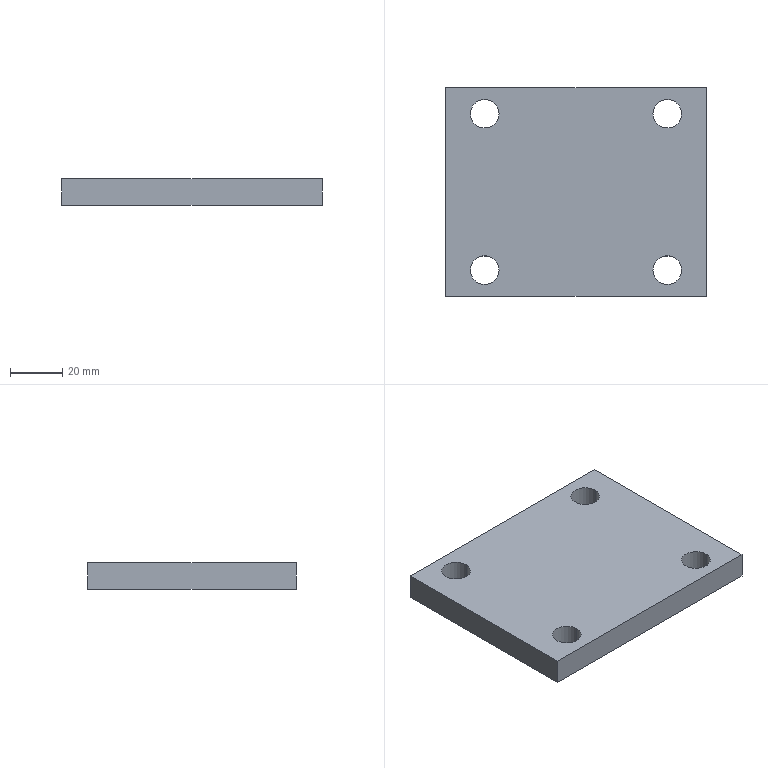Part | SolidWorks | features Extrusion 1 | 1 solid | 14 faces | box 100 x 80 x 10 mm | volume 76199 mm3 | cylinder 8 | plane 6 | commonest cylinder face diameters 11 x8
STEP:
#1=CARTESIAN_POINT('',(29.5,30.,10.));
#2=VERTEX_POINT('',#1);
#3=CARTESIAN_POINT('',(40.5,30.,10.));
#4=VERTEX_POINT('',#3);
#5=CARTESIAN_POINT('',(35.,30.,10.));
#6=DIRECTION('',(0.,0.,1.));
#7=DIRECTION('',(1.,0.,0.));
#8=AXIS2_PLACEMENT_3D('',#5,#6,#7);
#9=CIRCLE('',#8,5.5);
#10=EDGE_CURVE('',#2,#4,#9,.T.);
#11=ORIENTED_EDGE('',*,*,#10,.T.);
#12=CARTESIAN_POINT('',(40.5,30.,0.));
#13=VERTEX_POINT('',#12);
#14=CARTESIAN_POINT('',(40.5,30.,10.));
#15=DIRECTION('',(0.,0.,-1.));
#16=VECTOR('',#15,1000.);
#17=LINE('',#14,#16);
#18=EDGE_CURVE('',#4,#13,#17,.T.);
#19=ORIENTED_EDGE('',*,*,#18,.T.);
#20=CARTESIAN_POINT('',(29.5,30.,0.));
#21=VERTEX_POINT('',#20);
#22=CARTESIAN_POINT('',(35.,30.,0.));
#23=DIRECTION('',(0.,0.,1.));
#24=DIRECTION('',(1.,0.,0.));
#25=AXIS2_PLACEMENT_3D('',#22,#23,#24);
#26=CIRCLE('',#25,5.5);
#27=EDGE_CURVE('',#21,#13,#26,.T.);
#28=ORIENTED_EDGE('',*,*,#27,.F.);
#29=CARTESIAN_POINT('',(29.5,30.,10.));
#30=DIRECTION('',(0.,0.,-1.));
#31=VECTOR('',#30,1000.);
#32=LINE('',#29,#31);
#33=EDGE_CURVE('',#2,#21,#32,.T.);
#34=ORIENTED_EDGE('',*,*,#33,.F.);
#35=EDGE_LOOP('',(#11,#19,#28,#34));
#36=FACE_OUTER_BOUND('',#35,.T.);
#37=CARTESIAN_POINT('',(35.,30.,10.));
#38=DIRECTION('',(0.,0.,-1.));
#39=DIRECTION('',(-1.,0.,0.));
#40=AXIS2_PLACEMENT_3D('',#37,#38,#39);
#41=CYLINDRICAL_SURFACE('',#40,5.5);
#42=ADVANCED_FACE('',(#36),#41,.F.);
#43=CARTESIAN_POINT('',(29.5,-30.,10.));
#44=VERTEX_POINT('',#43);
#45=CARTESIAN_POINT('',(40.5,-30.,10.));
#46=VERTEX_POINT('',#45);
#47=CARTESIAN_POINT('',(35.,-30.,10.));
#48=DIRECTION('',(0.,0.,1.));
#49=DIRECTION('',(1.,0.,0.));
#50=AXIS2_PLACEMENT_3D('',#47,#48,#49);
#51=CIRCLE('',#50,5.5);
#52=EDGE_CURVE('',#44,#46,#51,.T.);
#53=ORIENTED_EDGE('',*,*,#52,.T.);
#54=CARTESIAN_POINT('',(40.5,-30.,0.));
#55=VERTEX_POINT('',#54);
#56=CARTESIAN_POINT('',(40.5,-30.,10.));
#57=DIRECTION('',(0.,0.,-1.));
#58=VECTOR('',#57,1000.);
#59=LINE('',#56,#58);
#60=EDGE_CURVE('',#46,#55,#59,.T.);
#61=ORIENTED_EDGE('',*,*,#60,.T.);
#62=CARTESIAN_POINT('',(29.5,-30.,0.));
#63=VERTEX_POINT('',#62);
#64=CARTESIAN_POINT('',(35.,-30.,0.));
#65=DIRECTION('',(0.,0.,1.));
#66=DIRECTION('',(1.,0.,0.));
#67=AXIS2_PLACEMENT_3D('',#64,#65,#66);
#68=CIRCLE('',#67,5.5);
#69=EDGE_CURVE('',#63,#55,#68,.T.);
#70=ORIENTED_EDGE('',*,*,#69,.F.);
#71=CARTESIAN_POINT('',(29.5,-30.,10.));
#72=DIRECTION('',(0.,0.,-1.));
#73=VECTOR('',#72,1000.);
#74=LINE('',#71,#73);
#75=EDGE_CURVE('',#44,#63,#74,.T.);
#76=ORIENTED_EDGE('',*,*,#75,.F.);
#77=EDGE_LOOP('',(#53,#61,#70,#76));
#78=FACE_OUTER_BOUND('',#77,.T.);
#79=CARTESIAN_POINT('',(35.,-30.,10.));
#80=DIRECTION('',(0.,0.,-1.));
#81=DIRECTION('',(-1.,0.,0.));
#82=AXIS2_PLACEMENT_3D('',#79,#80,#81);
#83=CYLINDRICAL_SURFACE('',#82,5.5);
#84=ADVANCED_FACE('',(#78),#83,.F.);
#85=CARTESIAN_POINT('',(-40.5,-30.,10.));
#86=VERTEX_POINT('',#85);
#87=CARTESIAN_POINT('',(-29.5,-30.,10.));
#88=VERTEX_POINT('',#87);
#89=CARTESIAN_POINT('',(-35.,-30.,10.));
#90=DIRECTION('',(0.,0.,1.));
#91=DIRECTION('',(1.,0.,0.));
#92=AXIS2_PLACEMENT_3D('',#89,#90,#91);
#93=CIRCLE('',#92,5.5);
#94=EDGE_CURVE('',#86,#88,#93,.T.);
#95=ORIENTED_EDGE('',*,*,#94,.T.);
#96=CARTESIAN_POINT('',(-29.5,-30.,0.));
#97=VERTEX_POINT('',#96);
#98=CARTESIAN_POINT('',(-29.5,-30.,10.));
#99=DIRECTION('',(0.,0.,-1.));
#100=VECTOR('',#99,1000.);
#101=LINE('',#98,#100);
#102=EDGE_CURVE('',#88,#97,#101,.T.);
#103=ORIENTED_EDGE('',*,*,#102,.T.);
#104=CARTESIAN_POINT('',(-40.5,-30.,0.));
#105=VERTEX_POINT('',#104);
#106=CARTESIAN_POINT('',(-35.,-30.,0.));
#107=DIRECTION('',(0.,0.,1.));
#108=DIRECTION('',(1.,0.,0.));
#109=AXIS2_PLACEMENT_3D('',#106,#107,#108);
#110=CIRCLE('',#109,5.5);
#111=EDGE_CURVE('',#105,#97,#110,.T.);
#112=ORIENTED_EDGE('',*,*,#111,.F.);
#113=CARTESIAN_POINT('',(-40.5,-30.,10.));
#114=DIRECTION('',(0.,0.,-1.));
#115=VECTOR('',#114,1000.);
#116=LINE('',#113,#115);
#117=EDGE_CURVE('',#86,#105,#116,.T.);
#118=ORIENTED_EDGE('',*,*,#117,.F.);
#119=EDGE_LOOP('',(#95,#103,#112,#118));
#120=FACE_OUTER_BOUND('',#119,.T.);
#121=CARTESIAN_POINT('',(-35.,-30.,10.));
#122=DIRECTION('',(0.,0.,-1.));
#123=DIRECTION('',(-1.,0.,0.));
#124=AXIS2_PLACEMENT_3D('',#121,#122,#123);
#125=CYLINDRICAL_SURFACE('',#124,5.5);
#126=ADVANCED_FACE('',(#120),#125,.F.);
#127=CARTESIAN_POINT('',(-40.5,30.,10.));
#128=VERTEX_POINT('',#127);
#129=CARTESIAN_POINT('',(-29.5,30.,10.));
#130=VERTEX_POINT('',#129);
#131=CARTESIAN_POINT('',(-35.,30.,10.));
#132=DIRECTION('',(0.,0.,1.));
#133=DIRECTION('',(1.,0.,0.));
#134=AXIS2_PLACEMENT_3D('',#131,#132,#133);
#135=CIRCLE('',#134,5.5);
#136=EDGE_CURVE('',#128,#130,#135,.T.);
#137=ORIENTED_EDGE('',*,*,#136,.T.);
#138=CARTESIAN_POINT('',(-29.5,30.,0.));
#139=VERTEX_POINT('',#138);
#140=CARTESIAN_POINT('',(-29.5,30.,10.));
#141=DIRECTION('',(0.,0.,-1.));
#142=VECTOR('',#141,1000.);
#143=LINE('',#140,#142);
#144=EDGE_CURVE('',#130,#139,#143,.T.);
#145=ORIENTED_EDGE('',*,*,#144,.T.);
#146=CARTESIAN_POINT('',(-40.5,30.,0.));
#147=VERTEX_POINT('',#146);
#148=CARTESIAN_POINT('',(-35.,30.,0.));
#149=DIRECTION('',(0.,0.,1.));
#150=DIRECTION('',(1.,0.,0.));
#151=AXIS2_PLACEMENT_3D('',#148,#149,#150);
#152=CIRCLE('',#151,5.5);
#153=EDGE_CURVE('',#147,#139,#152,.T.);
#154=ORIENTED_EDGE('',*,*,#153,.F.);
#155=CARTESIAN_POINT('',(-40.5,30.,10.));
#156=DIRECTION('',(0.,0.,-1.));
#157=VECTOR('',#156,1000.);
#158=LINE('',#155,#157);
#159=EDGE_CURVE('',#128,#147,#158,.T.);
#160=ORIENTED_EDGE('',*,*,#159,.F.);
#161=EDGE_LOOP('',(#137,#145,#154,#160));
#162=FACE_OUTER_BOUND('',#161,.T.);
#163=CARTESIAN_POINT('',(-35.,30.,10.));
#164=DIRECTION('',(0.,0.,-1.));
#165=DIRECTION('',(-1.,0.,0.));
#166=AXIS2_PLACEMENT_3D('',#163,#164,#165);
#167=CYLINDRICAL_SURFACE('',#166,5.5);
#168=ADVANCED_FACE('',(#162),#167,.F.);
#169=ORIENTED_EDGE('',*,*,#52,.F.);
#170=CARTESIAN_POINT('',(35.,-30.,10.));
#171=DIRECTION('',(0.,0.,1.));
#172=DIRECTION('',(1.,0.,0.));
#173=AXIS2_PLACEMENT_3D('',#170,#171,#172);
#174=CIRCLE('',#173,5.5);
#175=EDGE_CURVE('',#46,#44,#174,.T.);
#176=ORIENTED_EDGE('',*,*,#175,.F.);
#177=EDGE_LOOP('',(#169,#176));
#178=FACE_BOUND('',#177,.T.);
#179=ORIENTED_EDGE('',*,*,#136,.F.);
#180=CARTESIAN_POINT('',(-35.,30.,10.));
#181=DIRECTION('',(0.,0.,1.));
#182=DIRECTION('',(1.,0.,0.));
#183=AXIS2_PLACEMENT_3D('',#180,#181,#182);
#184=CIRCLE('',#183,5.5);
#185=EDGE_CURVE('',#130,#128,#184,.T.);
#186=ORIENTED_EDGE('',*,*,#185,.F.);
#187=EDGE_LOOP('',(#179,#186));
#188=FACE_BOUND('',#187,.T.);
#189=CARTESIAN_POINT('',(50.,-40.,10.));
#190=VERTEX_POINT('',#189);
#191=CARTESIAN_POINT('',(50.,40.,10.));
#192=VERTEX_POINT('',#191);
#193=CARTESIAN_POINT('',(50.,-40.,10.));
#194=DIRECTION('',(0.,1.,0.));
#195=VECTOR('',#194,1000.);
#196=LINE('',#193,#195);
#197=EDGE_CURVE('',#190,#192,#196,.T.);
#198=ORIENTED_EDGE('',*,*,#197,.T.);
#199=CARTESIAN_POINT('',(-50.,40.,10.));
#200=VERTEX_POINT('',#199);
#201=CARTESIAN_POINT('',(-50.,40.,10.));
#202=DIRECTION('',(-1.,0.,0.));
#203=VECTOR('',#202,1000.);
#204=LINE('',#201,#203);
#205=EDGE_CURVE('',#192,#200,#204,.T.);
#206=ORIENTED_EDGE('',*,*,#205,.T.);
#207=CARTESIAN_POINT('',(-50.,-40.,10.));
#208=VERTEX_POINT('',#207);
#209=CARTESIAN_POINT('',(-50.,-40.,10.));
#210=DIRECTION('',(0.,-1.,0.));
#211=VECTOR('',#210,1000.);
#212=LINE('',#209,#211);
#213=EDGE_CURVE('',#200,#208,#212,.T.);
#214=ORIENTED_EDGE('',*,*,#213,.T.);
#215=CARTESIAN_POINT('',(-50.,-40.,10.));
#216=DIRECTION('',(1.,0.,0.));
#217=VECTOR('',#216,1000.);
#218=LINE('',#215,#217);
#219=EDGE_CURVE('',#208,#190,#218,.T.);
#220=ORIENTED_EDGE('',*,*,#219,.T.);
#221=EDGE_LOOP('',(#198,#206,#214,#220));
#222=FACE_OUTER_BOUND('',#221,.T.);
#223=ORIENTED_EDGE('',*,*,#94,.F.);
#224=CARTESIAN_POINT('',(-35.,-30.,10.));
#225=DIRECTION('',(0.,0.,1.));
#226=DIRECTION('',(1.,0.,0.));
#227=AXIS2_PLACEMENT_3D('',#224,#225,#226);
#228=CIRCLE('',#227,5.5);
#229=EDGE_CURVE('',#88,#86,#228,.T.);
#230=ORIENTED_EDGE('',*,*,#229,.F.);
#231=EDGE_LOOP('',(#223,#230));
#232=FACE_BOUND('',#231,.T.);
#233=ORIENTED_EDGE('',*,*,#10,.F.);
#234=CARTESIAN_POINT('',(35.,30.,10.));
#235=DIRECTION('',(0.,0.,1.));
#236=DIRECTION('',(1.,0.,0.));
#237=AXIS2_PLACEMENT_3D('',#234,#235,#236);
#238=CIRCLE('',#237,5.5);
#239=EDGE_CURVE('',#4,#2,#238,.T.);
#240=ORIENTED_EDGE('',*,*,#239,.F.);
#241=EDGE_LOOP('',(#233,#240));
#242=FACE_BOUND('',#241,.T.);
#243=CARTESIAN_POINT('',(0.,0.,10.));
#244=DIRECTION('',(0.,0.,-1.));
#245=DIRECTION('',(-1.,0.,0.));
#246=AXIS2_PLACEMENT_3D('',#243,#244,#245);
#247=PLANE('',#246);
#248=ADVANCED_FACE('',(#178,#188,#222,#232,#242),#247,.F.);
#249=ORIENTED_EDGE('',*,*,#69,.T.);
#250=CARTESIAN_POINT('',(35.,-30.,0.));
#251=DIRECTION('',(0.,0.,1.));
#252=DIRECTION('',(1.,0.,0.));
#253=AXIS2_PLACEMENT_3D('',#250,#251,#252);
#254=CIRCLE('',#253,5.5);
#255=EDGE_CURVE('',#55,#63,#254,.T.);
#256=ORIENTED_EDGE('',*,*,#255,.T.);
#257=EDGE_LOOP('',(#249,#256));
#258=FACE_BOUND('',#257,.T.);
#259=ORIENTED_EDGE('',*,*,#153,.T.);
#260=CARTESIAN_POINT('',(-35.,30.,0.));
#261=DIRECTION('',(0.,0.,1.));
#262=DIRECTION('',(1.,0.,0.));
#263=AXIS2_PLACEMENT_3D('',#260,#261,#262);
#264=CIRCLE('',#263,5.5);
#265=EDGE_CURVE('',#139,#147,#264,.T.);
#266=ORIENTED_EDGE('',*,*,#265,.T.);
#267=EDGE_LOOP('',(#259,#266));
#268=FACE_BOUND('',#267,.T.);
#269=CARTESIAN_POINT('',(50.,-40.,0.));
#270=VERTEX_POINT('',#269);
#271=CARTESIAN_POINT('',(50.,40.,0.));
#272=VERTEX_POINT('',#271);
#273=CARTESIAN_POINT('',(50.,-40.,0.));
#274=DIRECTION('',(0.,1.,0.));
#275=VECTOR('',#274,1000.);
#276=LINE('',#273,#275);
#277=EDGE_CURVE('',#270,#272,#276,.T.);
#278=ORIENTED_EDGE('',*,*,#277,.F.);
#279=CARTESIAN_POINT('',(-50.,-40.,0.));
#280=VERTEX_POINT('',#279);
#281=CARTESIAN_POINT('',(-50.,-40.,0.));
#282=DIRECTION('',(1.,0.,0.));
#283=VECTOR('',#282,1000.);
#284=LINE('',#281,#283);
#285=EDGE_CURVE('',#280,#270,#284,.T.);
#286=ORIENTED_EDGE('',*,*,#285,.F.);
#287=CARTESIAN_POINT('',(-50.,40.,0.));
#288=VERTEX_POINT('',#287);
#289=CARTESIAN_POINT('',(-50.,-40.,0.));
#290=DIRECTION('',(0.,-1.,0.));
#291=VECTOR('',#290,1000.);
#292=LINE('',#289,#291);
#293=EDGE_CURVE('',#288,#280,#292,.T.);
#294=ORIENTED_EDGE('',*,*,#293,.F.);
#295=CARTESIAN_POINT('',(-50.,40.,0.));
#296=DIRECTION('',(-1.,0.,0.));
#297=VECTOR('',#296,1000.);
#298=LINE('',#295,#297);
#299=EDGE_CURVE('',#272,#288,#298,.T.);
#300=ORIENTED_EDGE('',*,*,#299,.F.);
#301=EDGE_LOOP('',(#278,#286,#294,#300));
#302=FACE_OUTER_BOUND('',#301,.T.);
#303=ORIENTED_EDGE('',*,*,#111,.T.);
#304=CARTESIAN_POINT('',(-35.,-30.,0.));
#305=DIRECTION('',(0.,0.,1.));
#306=DIRECTION('',(1.,0.,0.));
#307=AXIS2_PLACEMENT_3D('',#304,#305,#306);
#308=CIRCLE('',#307,5.5);
#309=EDGE_CURVE('',#97,#105,#308,.T.);
#310=ORIENTED_EDGE('',*,*,#309,.T.);
#311=EDGE_LOOP('',(#303,#310));
#312=FACE_BOUND('',#311,.T.);
#313=ORIENTED_EDGE('',*,*,#27,.T.);
#314=CARTESIAN_POINT('',(35.,30.,0.));
#315=DIRECTION('',(0.,0.,1.));
#316=DIRECTION('',(1.,0.,0.));
#317=AXIS2_PLACEMENT_3D('',#314,#315,#316);
#318=CIRCLE('',#317,5.5);
#319=EDGE_CURVE('',#13,#21,#318,.T.);
#320=ORIENTED_EDGE('',*,*,#319,.T.);
#321=EDGE_LOOP('',(#313,#320));
#322=FACE_BOUND('',#321,.T.);
#323=CARTESIAN_POINT('',(0.,0.,0.));
#324=DIRECTION('',(0.,0.,-1.));
#325=DIRECTION('',(-1.,0.,0.));
#326=AXIS2_PLACEMENT_3D('',#323,#324,#325);
#327=PLANE('',#326);
#328=ADVANCED_FACE('',(#258,#268,#302,#312,#322),#327,.T.);
#329=ORIENTED_EDGE('',*,*,#277,.T.);
#330=CARTESIAN_POINT('',(50.,40.,10.));
#331=DIRECTION('',(0.,0.,-1.));
#332=VECTOR('',#331,1000.);
#333=LINE('',#330,#332);
#334=EDGE_CURVE('',#192,#272,#333,.T.);
#335=ORIENTED_EDGE('',*,*,#334,.F.);
#336=ORIENTED_EDGE('',*,*,#197,.F.);
#337=CARTESIAN_POINT('',(50.,-40.,10.));
#338=DIRECTION('',(0.,0.,-1.));
#339=VECTOR('',#338,1000.);
#340=LINE('',#337,#339);
#341=EDGE_CURVE('',#190,#270,#340,.T.);
#342=ORIENTED_EDGE('',*,*,#341,.T.);
#343=EDGE_LOOP('',(#329,#335,#336,#342));
#344=FACE_OUTER_BOUND('',#343,.T.);
#345=CARTESIAN_POINT('',(50.,-40.,10.));
#346=DIRECTION('',(-1.,0.,0.));
#347=DIRECTION('',(0.,0.,1.));
#348=AXIS2_PLACEMENT_3D('',#345,#346,#347);
#349=PLANE('',#348);
#350=ADVANCED_FACE('',(#344),#349,.F.);
#351=ORIENTED_EDGE('',*,*,#299,.T.);
#352=CARTESIAN_POINT('',(-50.,40.,10.));
#353=DIRECTION('',(0.,0.,-1.));
#354=VECTOR('',#353,1000.);
#355=LINE('',#352,#354);
#356=EDGE_CURVE('',#200,#288,#355,.T.);
#357=ORIENTED_EDGE('',*,*,#356,.F.);
#358=ORIENTED_EDGE('',*,*,#205,.F.);
#359=ORIENTED_EDGE('',*,*,#334,.T.);
#360=EDGE_LOOP('',(#351,#357,#358,#359));
#361=FACE_OUTER_BOUND('',#360,.T.);
#362=CARTESIAN_POINT('',(-50.,40.,10.));
#363=DIRECTION('',(0.,-1.,0.));
#364=DIRECTION('',(0.,0.,-1.));
#365=AXIS2_PLACEMENT_3D('',#362,#363,#364);
#366=PLANE('',#365);
#367=ADVANCED_FACE('',(#361),#366,.F.);
#368=ORIENTED_EDGE('',*,*,#293,.T.);
#369=CARTESIAN_POINT('',(-50.,-40.,10.));
#370=DIRECTION('',(0.,0.,-1.));
#371=VECTOR('',#370,1000.);
#372=LINE('',#369,#371);
#373=EDGE_CURVE('',#208,#280,#372,.T.);
#374=ORIENTED_EDGE('',*,*,#373,.F.);
#375=ORIENTED_EDGE('',*,*,#213,.F.);
#376=ORIENTED_EDGE('',*,*,#356,.T.);
#377=EDGE_LOOP('',(#368,#374,#375,#376));
#378=FACE_OUTER_BOUND('',#377,.T.);
#379=CARTESIAN_POINT('',(-50.,-40.,10.));
#380=DIRECTION('',(1.,0.,0.));
#381=DIRECTION('',(0.,0.,-1.));
#382=AXIS2_PLACEMENT_3D('',#379,#380,#381);
#383=PLANE('',#382);
#384=ADVANCED_FACE('',(#378),#383,.F.);
#385=ORIENTED_EDGE('',*,*,#285,.T.);
#386=ORIENTED_EDGE('',*,*,#341,.F.);
#387=ORIENTED_EDGE('',*,*,#219,.F.);
#388=ORIENTED_EDGE('',*,*,#373,.T.);
#389=EDGE_LOOP('',(#385,#386,#387,#388));
#390=FACE_OUTER_BOUND('',#389,.T.);
#391=CARTESIAN_POINT('',(-50.,-40.,10.));
#392=DIRECTION('',(0.,1.,0.));
#393=DIRECTION('',(0.,0.,1.));
#394=AXIS2_PLACEMENT_3D('',#391,#392,#393);
#395=PLANE('',#394);
#396=ADVANCED_FACE('',(#390),#395,.F.);
#397=ORIENTED_EDGE('',*,*,#144,.F.);
#398=ORIENTED_EDGE('',*,*,#185,.T.);
#399=ORIENTED_EDGE('',*,*,#159,.T.);
#400=ORIENTED_EDGE('',*,*,#265,.F.);
#401=EDGE_LOOP('',(#397,#398,#399,#400));
#402=FACE_OUTER_BOUND('',#401,.T.);
#403=CARTESIAN_POINT('',(-35.,30.,10.));
#404=DIRECTION('',(0.,0.,-1.));
#405=DIRECTION('',(-1.,0.,0.));
#406=AXIS2_PLACEMENT_3D('',#403,#404,#405);
#407=CYLINDRICAL_SURFACE('',#406,5.5);
#408=ADVANCED_FACE('',(#402),#407,.F.);
#409=ORIENTED_EDGE('',*,*,#102,.F.);
#410=ORIENTED_EDGE('',*,*,#229,.T.);
#411=ORIENTED_EDGE('',*,*,#117,.T.);
#412=ORIENTED_EDGE('',*,*,#309,.F.);
#413=EDGE_LOOP('',(#409,#410,#411,#412));
#414=FACE_OUTER_BOUND('',#413,.T.);
#415=CARTESIAN_POINT('',(-35.,-30.,10.));
#416=DIRECTION('',(0.,0.,-1.));
#417=DIRECTION('',(-1.,0.,0.));
#418=AXIS2_PLACEMENT_3D('',#415,#416,#417);
#419=CYLINDRICAL_SURFACE('',#418,5.5);
#420=ADVANCED_FACE('',(#414),#419,.F.);
#421=ORIENTED_EDGE('',*,*,#60,.F.);
#422=ORIENTED_EDGE('',*,*,#175,.T.);
#423=ORIENTED_EDGE('',*,*,#75,.T.);
#424=ORIENTED_EDGE('',*,*,#255,.F.);
#425=EDGE_LOOP('',(#421,#422,#423,#424));
#426=FACE_OUTER_BOUND('',#425,.T.);
#427=CARTESIAN_POINT('',(35.,-30.,10.));
#428=DIRECTION('',(0.,0.,-1.));
#429=DIRECTION('',(-1.,0.,0.));
#430=AXIS2_PLACEMENT_3D('',#427,#428,#429);
#431=CYLINDRICAL_SURFACE('',#430,5.5);
#432=ADVANCED_FACE('',(#426),#431,.F.);
#433=ORIENTED_EDGE('',*,*,#18,.F.);
#434=ORIENTED_EDGE('',*,*,#239,.T.);
#435=ORIENTED_EDGE('',*,*,#33,.T.);
#436=ORIENTED_EDGE('',*,*,#319,.F.);
#437=EDGE_LOOP('',(#433,#434,#435,#436));
#438=FACE_OUTER_BOUND('',#437,.T.);
#439=CARTESIAN_POINT('',(35.,30.,10.));
#440=DIRECTION('',(0.,0.,-1.));
#441=DIRECTION('',(-1.,0.,0.));
#442=AXIS2_PLACEMENT_3D('',#439,#440,#441);
#443=CYLINDRICAL_SURFACE('',#442,5.5);
#444=ADVANCED_FACE('',(#438),#443,.F.);
#445=CLOSED_SHELL('',(#42,#84,#126,#168,#248,#328,#350,#367,#384,#396,#408,#420,#432,#444));
#446=MANIFOLD_SOLID_BREP('',#445);
#447=CARTESIAN_POINT('',(0.,0.,0.));
#448=DIRECTION('',(0.,0.,1.));
#449=DIRECTION('',(1.,0.,0.));
#450=AXIS2_PLACEMENT_3D('',#447,#448,#449);
#451=(LENGTH_UNIT()NAMED_UNIT(*)SI_UNIT(.MILLI.,.METRE.));
#452=UNCERTAINTY_MEASURE_WITH_UNIT(LENGTH_MEASURE(0.00001),#451,'','');
#453=(NAMED_UNIT(*)PLANE_ANGLE_UNIT()SI_UNIT($,.RADIAN.));
#454=(NAMED_UNIT(*)SI_UNIT($,.STERADIAN.)SOLID_ANGLE_UNIT());
#455=(GEOMETRIC_REPRESENTATION_CONTEXT(3)GLOBAL_UNCERTAINTY_ASSIGNED_CONTEXT((#452))GLOBAL_UNIT_ASSIGNED_CONTEXT((#451,#453,#454))REPRESENTATION_CONTEXT('',''));
#456=ADVANCED_BREP_SHAPE_REPRESENTATION('',(#446,#450),#455);